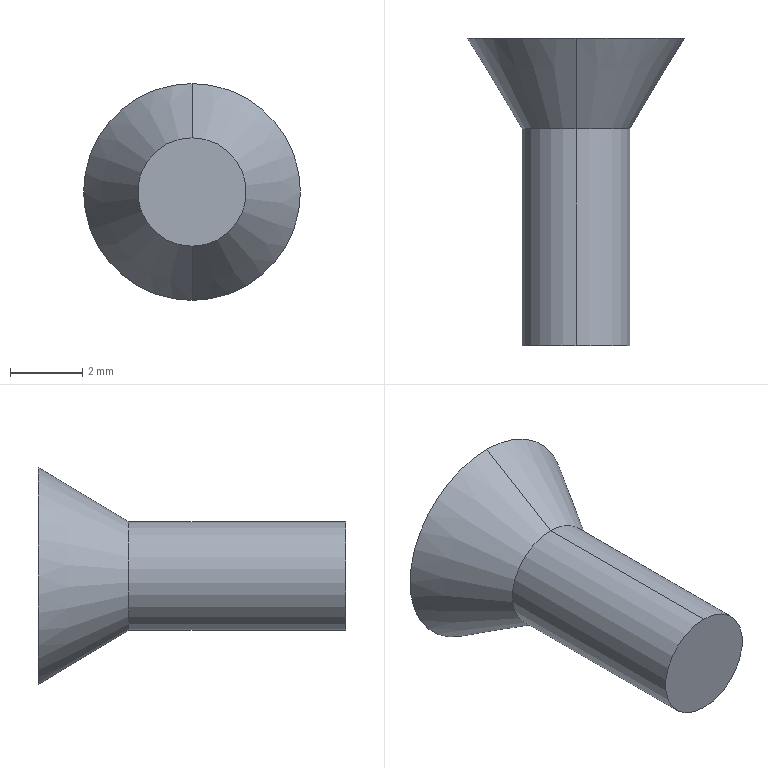Part | SolidWorks | features BaseBody 1 | 1 solid | 13 faces | box 6 x 8.5 x 6 mm | volume 80.181 mm3 | plane 9 | cylinder 2 | cone 2 | commonest cylinder face diameters 3 x2
STEP:
#1=CARTESIAN_POINT('',(3.272,-8.5,1.5));
#2=VERTEX_POINT('',#1);
#3=CARTESIAN_POINT('',(3.272,-8.5,-1.5));
#4=VERTEX_POINT('',#3);
#5=CARTESIAN_POINT('',(3.272,-8.5,0.));
#6=DIRECTION('',(0.,1.,0.));
#7=DIRECTION('',(0.,0.,1.));
#8=AXIS2_PLACEMENT_3D('',#5,#6,#7);
#9=CIRCLE('',#8,1.5);
#10=EDGE_CURVE('',#2,#4,#9,.T.);
#11=ORIENTED_EDGE('',*,*,#10,.T.);
#12=CARTESIAN_POINT('',(3.272,-2.5,-1.5));
#13=VERTEX_POINT('',#12);
#14=CARTESIAN_POINT('',(3.272,-8.5,-1.5));
#15=DIRECTION('',(0.,1.,0.));
#16=VECTOR('',#15,1000.);
#17=LINE('',#14,#16);
#18=EDGE_CURVE('',#4,#13,#17,.T.);
#19=ORIENTED_EDGE('',*,*,#18,.T.);
#20=CARTESIAN_POINT('',(3.272,-2.5,1.5));
#21=VERTEX_POINT('',#20);
#22=CARTESIAN_POINT('',(3.272,-2.5,0.));
#23=DIRECTION('',(0.,-1.,0.));
#24=DIRECTION('',(0.,0.,1.));
#25=AXIS2_PLACEMENT_3D('',#22,#23,#24);
#26=CIRCLE('',#25,1.5);
#27=EDGE_CURVE('',#13,#21,#26,.T.);
#28=ORIENTED_EDGE('',*,*,#27,.T.);
#29=CARTESIAN_POINT('',(3.272,-8.5,1.5));
#30=DIRECTION('',(0.,1.,0.));
#31=VECTOR('',#30,1000.);
#32=LINE('',#29,#31);
#33=EDGE_CURVE('',#2,#21,#32,.T.);
#34=ORIENTED_EDGE('',*,*,#33,.F.);
#35=EDGE_LOOP('',(#11,#19,#28,#34));
#36=FACE_OUTER_BOUND('',#35,.T.);
#37=CARTESIAN_POINT('',(3.272,-8.5,0.));
#38=DIRECTION('',(0.,1.,0.));
#39=DIRECTION('',(0.,0.,1.));
#40=AXIS2_PLACEMENT_3D('',#37,#38,#39);
#41=CYLINDRICAL_SURFACE('',#40,1.5);
#42=ADVANCED_FACE('',(#36),#41,.T.);
#43=ORIENTED_EDGE('',*,*,#27,.F.);
#44=CARTESIAN_POINT('',(3.272,0.,-3.));
#45=VERTEX_POINT('',#44);
#46=CARTESIAN_POINT('',(3.272,0.,-3.));
#47=DIRECTION('',(0.,0.8575,-0.5145));
#48=VECTOR('',#47,1000.);
#49=LINE('',#46,#48);
#50=EDGE_CURVE('',#13,#45,#49,.T.);
#51=ORIENTED_EDGE('',*,*,#50,.T.);
#52=CARTESIAN_POINT('',(3.272,0.,3.));
#53=VERTEX_POINT('',#52);
#54=CARTESIAN_POINT('',(3.272,0.,0.));
#55=DIRECTION('',(0.,-1.,0.));
#56=DIRECTION('',(0.,0.,1.));
#57=AXIS2_PLACEMENT_3D('',#54,#55,#56);
#58=CIRCLE('',#57,3.);
#59=EDGE_CURVE('',#45,#53,#58,.T.);
#60=ORIENTED_EDGE('',*,*,#59,.T.);
#61=CARTESIAN_POINT('',(3.272,0.,3.));
#62=DIRECTION('',(0.,0.8575,0.5145));
#63=VECTOR('',#62,1000.);
#64=LINE('',#61,#63);
#65=EDGE_CURVE('',#21,#53,#64,.T.);
#66=ORIENTED_EDGE('',*,*,#65,.F.);
#67=EDGE_LOOP('',(#43,#51,#60,#66));
#68=FACE_OUTER_BOUND('',#67,.T.);
#69=CARTESIAN_POINT('',(3.272,0.,0.));
#70=DIRECTION('',(0.,1.,0.));
#71=DIRECTION('',(0.,0.,1.));
#72=AXIS2_PLACEMENT_3D('',#69,#70,#71);
#73=CONICAL_SURFACE('',#72,3.,0.5404);
#74=ADVANCED_FACE('',(#68),#73,.T.);
#75=ORIENTED_EDGE('',*,*,#18,.F.);
#76=CARTESIAN_POINT('',(3.272,-8.5,0.));
#77=DIRECTION('',(0.,1.,0.));
#78=DIRECTION('',(0.,0.,1.));
#79=AXIS2_PLACEMENT_3D('',#76,#77,#78);
#80=CIRCLE('',#79,1.5);
#81=EDGE_CURVE('',#4,#2,#80,.T.);
#82=ORIENTED_EDGE('',*,*,#81,.T.);
#83=ORIENTED_EDGE('',*,*,#33,.T.);
#84=CARTESIAN_POINT('',(3.272,-2.5,0.));
#85=DIRECTION('',(0.,-1.,0.));
#86=DIRECTION('',(0.,0.,1.));
#87=AXIS2_PLACEMENT_3D('',#84,#85,#86);
#88=CIRCLE('',#87,1.5);
#89=EDGE_CURVE('',#21,#13,#88,.T.);
#90=ORIENTED_EDGE('',*,*,#89,.T.);
#91=EDGE_LOOP('',(#75,#82,#83,#90));
#92=FACE_OUTER_BOUND('',#91,.T.);
#93=CARTESIAN_POINT('',(3.272,-8.5,0.));
#94=DIRECTION('',(0.,1.,0.));
#95=DIRECTION('',(0.,0.,1.));
#96=AXIS2_PLACEMENT_3D('',#93,#94,#95);
#97=CYLINDRICAL_SURFACE('',#96,1.5);
#98=ADVANCED_FACE('',(#92),#97,.T.);
#99=ORIENTED_EDGE('',*,*,#50,.F.);
#100=ORIENTED_EDGE('',*,*,#89,.F.);
#101=ORIENTED_EDGE('',*,*,#65,.T.);
#102=CARTESIAN_POINT('',(3.272,0.,0.));
#103=DIRECTION('',(0.,-1.,0.));
#104=DIRECTION('',(0.,0.,1.));
#105=AXIS2_PLACEMENT_3D('',#102,#103,#104);
#106=CIRCLE('',#105,3.);
#107=EDGE_CURVE('',#53,#45,#106,.T.);
#108=ORIENTED_EDGE('',*,*,#107,.T.);
#109=EDGE_LOOP('',(#99,#100,#101,#108));
#110=FACE_OUTER_BOUND('',#109,.T.);
#111=CARTESIAN_POINT('',(3.272,0.,0.));
#112=DIRECTION('',(0.,1.,0.));
#113=DIRECTION('',(0.,0.,1.));
#114=AXIS2_PLACEMENT_3D('',#111,#112,#113);
#115=CONICAL_SURFACE('',#114,3.,0.5404);
#116=ADVANCED_FACE('',(#110),#115,.T.);
#117=ORIENTED_EDGE('',*,*,#10,.F.);
#118=ORIENTED_EDGE('',*,*,#81,.F.);
#119=EDGE_LOOP('',(#117,#118));
#120=FACE_OUTER_BOUND('',#119,.T.);
#121=CARTESIAN_POINT('',(3.272,-8.5,0.));
#122=DIRECTION('',(0.,-1.,0.));
#123=DIRECTION('',(0.,0.,-1.));
#124=AXIS2_PLACEMENT_3D('',#121,#122,#123);
#125=PLANE('',#124);
#126=ADVANCED_FACE('',(#120),#125,.T.);
#127=ORIENTED_EDGE('',*,*,#107,.F.);
#128=ORIENTED_EDGE('',*,*,#59,.F.);
#129=EDGE_LOOP('',(#127,#128));
#130=FACE_OUTER_BOUND('',#129,.T.);
#131=CARTESIAN_POINT('',(2.695,0.,-1.));
#132=VERTEX_POINT('',#131);
#133=CARTESIAN_POINT('',(3.85,0.,-1.));
#134=VERTEX_POINT('',#133);
#135=CARTESIAN_POINT('',(3.272,0.,-1.));
#136=DIRECTION('',(1.,0.,0.));
#137=VECTOR('',#136,1000.);
#138=LINE('',#135,#137);
#139=EDGE_CURVE('',#132,#134,#138,.T.);
#140=ORIENTED_EDGE('',*,*,#139,.T.);
#141=CARTESIAN_POINT('',(4.427,0.,0.));
#142=VERTEX_POINT('',#141);
#143=CARTESIAN_POINT('',(3.85,0.,-1.));
#144=DIRECTION('',(0.5,0.,0.866));
#145=VECTOR('',#144,1000.);
#146=LINE('',#143,#145);
#147=EDGE_CURVE('',#134,#142,#146,.T.);
#148=ORIENTED_EDGE('',*,*,#147,.T.);
#149=CARTESIAN_POINT('',(3.85,0.,1.));
#150=VERTEX_POINT('',#149);
#151=CARTESIAN_POINT('',(4.427,0.,0.));
#152=DIRECTION('',(-0.5,0.,0.866));
#153=VECTOR('',#152,1000.);
#154=LINE('',#151,#153);
#155=EDGE_CURVE('',#142,#150,#154,.T.);
#156=ORIENTED_EDGE('',*,*,#155,.T.);
#157=CARTESIAN_POINT('',(2.695,0.,1.));
#158=VERTEX_POINT('',#157);
#159=CARTESIAN_POINT('',(3.272,0.,1.));
#160=DIRECTION('',(-1.,0.,0.));
#161=VECTOR('',#160,1000.);
#162=LINE('',#159,#161);
#163=EDGE_CURVE('',#150,#158,#162,.T.);
#164=ORIENTED_EDGE('',*,*,#163,.T.);
#165=CARTESIAN_POINT('',(2.118,0.,0.));
#166=VERTEX_POINT('',#165);
#167=CARTESIAN_POINT('',(2.695,0.,1.));
#168=DIRECTION('',(-0.5,0.,-0.866));
#169=VECTOR('',#168,1000.);
#170=LINE('',#167,#169);
#171=EDGE_CURVE('',#158,#166,#170,.T.);
#172=ORIENTED_EDGE('',*,*,#171,.T.);
#173=CARTESIAN_POINT('',(2.118,0.,0.));
#174=DIRECTION('',(0.5,0.,-0.866));
#175=VECTOR('',#174,1000.);
#176=LINE('',#173,#175);
#177=EDGE_CURVE('',#166,#132,#176,.T.);
#178=ORIENTED_EDGE('',*,*,#177,.T.);
#179=EDGE_LOOP('',(#140,#148,#156,#164,#172,#178));
#180=FACE_BOUND('',#179,.T.);
#181=CARTESIAN_POINT('',(3.272,0.,0.));
#182=DIRECTION('',(0.,1.,0.));
#183=DIRECTION('',(0.,0.,1.));
#184=AXIS2_PLACEMENT_3D('',#181,#182,#183);
#185=PLANE('',#184);
#186=ADVANCED_FACE('',(#130,#180),#185,.T.);
#187=CARTESIAN_POINT('',(3.85,-1.,-1.));
#188=VERTEX_POINT('',#187);
#189=CARTESIAN_POINT('',(3.85,-1.,-1.));
#190=DIRECTION('',(0.,1.,0.));
#191=VECTOR('',#190,1000.);
#192=LINE('',#189,#191);
#193=EDGE_CURVE('',#188,#134,#192,.T.);
#194=ORIENTED_EDGE('',*,*,#193,.F.);
#195=CARTESIAN_POINT('',(4.427,-1.,0.));
#196=VERTEX_POINT('',#195);
#197=CARTESIAN_POINT('',(4.427,-1.,0.));
#198=DIRECTION('',(-0.5,0.,-0.866));
#199=VECTOR('',#198,1000.);
#200=LINE('',#197,#199);
#201=EDGE_CURVE('',#196,#188,#200,.T.);
#202=ORIENTED_EDGE('',*,*,#201,.F.);
#203=CARTESIAN_POINT('',(4.427,-1.,0.));
#204=DIRECTION('',(0.,-1.,0.));
#205=VECTOR('',#204,1000.);
#206=LINE('',#203,#205);
#207=EDGE_CURVE('',#142,#196,#206,.T.);
#208=ORIENTED_EDGE('',*,*,#207,.F.);
#209=ORIENTED_EDGE('',*,*,#147,.F.);
#210=EDGE_LOOP('',(#194,#202,#208,#209));
#211=FACE_OUTER_BOUND('',#210,.T.);
#212=CARTESIAN_POINT('',(4.427,-1.,0.));
#213=DIRECTION('',(0.866,0.,-0.5));
#214=DIRECTION('',(-0.5,0.,-0.866));
#215=AXIS2_PLACEMENT_3D('',#212,#213,#214);
#216=PLANE('',#215);
#217=ADVANCED_FACE('',(#211),#216,.F.);
#218=CARTESIAN_POINT('',(2.695,-1.,-1.));
#219=VERTEX_POINT('',#218);
#220=CARTESIAN_POINT('',(2.695,-1.,-1.));
#221=DIRECTION('',(0.,1.,0.));
#222=VECTOR('',#221,1000.);
#223=LINE('',#220,#222);
#224=EDGE_CURVE('',#219,#132,#223,.T.);
#225=ORIENTED_EDGE('',*,*,#224,.F.);
#226=CARTESIAN_POINT('',(3.85,-1.,-1.));
#227=DIRECTION('',(-1.,0.,0.));
#228=VECTOR('',#227,1000.);
#229=LINE('',#226,#228);
#230=EDGE_CURVE('',#188,#219,#229,.T.);
#231=ORIENTED_EDGE('',*,*,#230,.F.);
#232=ORIENTED_EDGE('',*,*,#193,.T.);
#233=ORIENTED_EDGE('',*,*,#139,.F.);
#234=EDGE_LOOP('',(#225,#231,#232,#233));
#235=FACE_OUTER_BOUND('',#234,.T.);
#236=CARTESIAN_POINT('',(3.85,-1.,-1.));
#237=DIRECTION('',(0.,0.,-1.));
#238=DIRECTION('',(-1.,0.,0.));
#239=AXIS2_PLACEMENT_3D('',#236,#237,#238);
#240=PLANE('',#239);
#241=ADVANCED_FACE('',(#235),#240,.F.);
#242=CARTESIAN_POINT('',(2.118,-1.,0.));
#243=VERTEX_POINT('',#242);
#244=CARTESIAN_POINT('',(2.118,-1.,0.));
#245=DIRECTION('',(0.,1.,0.));
#246=VECTOR('',#245,1000.);
#247=LINE('',#244,#246);
#248=EDGE_CURVE('',#243,#166,#247,.T.);
#249=ORIENTED_EDGE('',*,*,#248,.F.);
#250=CARTESIAN_POINT('',(2.695,-1.,-1.));
#251=DIRECTION('',(-0.5,0.,0.866));
#252=VECTOR('',#251,1000.);
#253=LINE('',#250,#252);
#254=EDGE_CURVE('',#219,#243,#253,.T.);
#255=ORIENTED_EDGE('',*,*,#254,.F.);
#256=ORIENTED_EDGE('',*,*,#224,.T.);
#257=ORIENTED_EDGE('',*,*,#177,.F.);
#258=EDGE_LOOP('',(#249,#255,#256,#257));
#259=FACE_OUTER_BOUND('',#258,.T.);
#260=CARTESIAN_POINT('',(2.695,-1.,-1.));
#261=DIRECTION('',(-0.866,0.,-0.5));
#262=DIRECTION('',(-0.5,0.,0.866));
#263=AXIS2_PLACEMENT_3D('',#260,#261,#262);
#264=PLANE('',#263);
#265=ADVANCED_FACE('',(#259),#264,.F.);
#266=CARTESIAN_POINT('',(2.695,-1.,1.));
#267=VERTEX_POINT('',#266);
#268=CARTESIAN_POINT('',(2.695,-1.,1.));
#269=DIRECTION('',(0.,1.,0.));
#270=VECTOR('',#269,1000.);
#271=LINE('',#268,#270);
#272=EDGE_CURVE('',#267,#158,#271,.T.);
#273=ORIENTED_EDGE('',*,*,#272,.F.);
#274=CARTESIAN_POINT('',(2.118,-1.,0.));
#275=DIRECTION('',(0.5,0.,0.866));
#276=VECTOR('',#275,1000.);
#277=LINE('',#274,#276);
#278=EDGE_CURVE('',#243,#267,#277,.T.);
#279=ORIENTED_EDGE('',*,*,#278,.F.);
#280=ORIENTED_EDGE('',*,*,#248,.T.);
#281=ORIENTED_EDGE('',*,*,#171,.F.);
#282=EDGE_LOOP('',(#273,#279,#280,#281));
#283=FACE_OUTER_BOUND('',#282,.T.);
#284=CARTESIAN_POINT('',(2.118,-1.,0.));
#285=DIRECTION('',(-0.866,0.,0.5));
#286=DIRECTION('',(0.5,0.,0.866));
#287=AXIS2_PLACEMENT_3D('',#284,#285,#286);
#288=PLANE('',#287);
#289=ADVANCED_FACE('',(#283),#288,.F.);
#290=CARTESIAN_POINT('',(3.85,-1.,1.));
#291=VERTEX_POINT('',#290);
#292=CARTESIAN_POINT('',(3.85,-1.,1.));
#293=DIRECTION('',(0.,1.,0.));
#294=VECTOR('',#293,1000.);
#295=LINE('',#292,#294);
#296=EDGE_CURVE('',#291,#150,#295,.T.);
#297=ORIENTED_EDGE('',*,*,#296,.F.);
#298=CARTESIAN_POINT('',(2.695,-1.,1.));
#299=DIRECTION('',(1.,0.,0.));
#300=VECTOR('',#299,1000.);
#301=LINE('',#298,#300);
#302=EDGE_CURVE('',#267,#291,#301,.T.);
#303=ORIENTED_EDGE('',*,*,#302,.F.);
#304=ORIENTED_EDGE('',*,*,#272,.T.);
#305=ORIENTED_EDGE('',*,*,#163,.F.);
#306=EDGE_LOOP('',(#297,#303,#304,#305));
#307=FACE_OUTER_BOUND('',#306,.T.);
#308=CARTESIAN_POINT('',(2.695,-1.,1.));
#309=DIRECTION('',(0.,0.,1.));
#310=DIRECTION('',(1.,0.,0.));
#311=AXIS2_PLACEMENT_3D('',#308,#309,#310);
#312=PLANE('',#311);
#313=ADVANCED_FACE('',(#307),#312,.F.);
#314=ORIENTED_EDGE('',*,*,#207,.T.);
#315=CARTESIAN_POINT('',(3.85,-1.,1.));
#316=DIRECTION('',(0.5,0.,-0.866));
#317=VECTOR('',#316,1000.);
#318=LINE('',#315,#317);
#319=EDGE_CURVE('',#291,#196,#318,.T.);
#320=ORIENTED_EDGE('',*,*,#319,.F.);
#321=ORIENTED_EDGE('',*,*,#296,.T.);
#322=ORIENTED_EDGE('',*,*,#155,.F.);
#323=EDGE_LOOP('',(#314,#320,#321,#322));
#324=FACE_OUTER_BOUND('',#323,.T.);
#325=CARTESIAN_POINT('',(3.85,-1.,1.));
#326=DIRECTION('',(0.866,0.,0.5));
#327=DIRECTION('',(0.5,0.,-0.866));
#328=AXIS2_PLACEMENT_3D('',#325,#326,#327);
#329=PLANE('',#328);
#330=ADVANCED_FACE('',(#324),#329,.F.);
#331=ORIENTED_EDGE('',*,*,#278,.T.);
#332=ORIENTED_EDGE('',*,*,#302,.T.);
#333=ORIENTED_EDGE('',*,*,#319,.T.);
#334=ORIENTED_EDGE('',*,*,#201,.T.);
#335=ORIENTED_EDGE('',*,*,#230,.T.);
#336=ORIENTED_EDGE('',*,*,#254,.T.);
#337=EDGE_LOOP('',(#331,#332,#333,#334,#335,#336));
#338=FACE_OUTER_BOUND('',#337,.T.);
#339=CARTESIAN_POINT('',(0.,-1.,0.));
#340=DIRECTION('',(0.,1.,0.));
#341=DIRECTION('',(0.,0.,1.));
#342=AXIS2_PLACEMENT_3D('',#339,#340,#341);
#343=PLANE('',#342);
#344=ADVANCED_FACE('',(#338),#343,.T.);
#345=CLOSED_SHELL('',(#42,#74,#98,#116,#126,#186,#217,#241,#265,#289,#313,#330,#344));
#346=MANIFOLD_SOLID_BREP('',#345);
#347=CARTESIAN_POINT('',(0.,0.,0.));
#348=DIRECTION('',(0.,0.,1.));
#349=DIRECTION('',(1.,0.,0.));
#350=AXIS2_PLACEMENT_3D('',#347,#348,#349);
#351=(LENGTH_UNIT()NAMED_UNIT(*)SI_UNIT(.MILLI.,.METRE.));
#352=UNCERTAINTY_MEASURE_WITH_UNIT(LENGTH_MEASURE(0.00001),#351,'','');
#353=(NAMED_UNIT(*)PLANE_ANGLE_UNIT()SI_UNIT($,.RADIAN.));
#354=(NAMED_UNIT(*)SI_UNIT($,.STERADIAN.)SOLID_ANGLE_UNIT());
#355=(GEOMETRIC_REPRESENTATION_CONTEXT(3)GLOBAL_UNCERTAINTY_ASSIGNED_CONTEXT((#352))GLOBAL_UNIT_ASSIGNED_CONTEXT((#351,#353,#354))REPRESENTATION_CONTEXT('',''));
#356=ADVANCED_BREP_SHAPE_REPRESENTATION('',(#346,#350),#355);